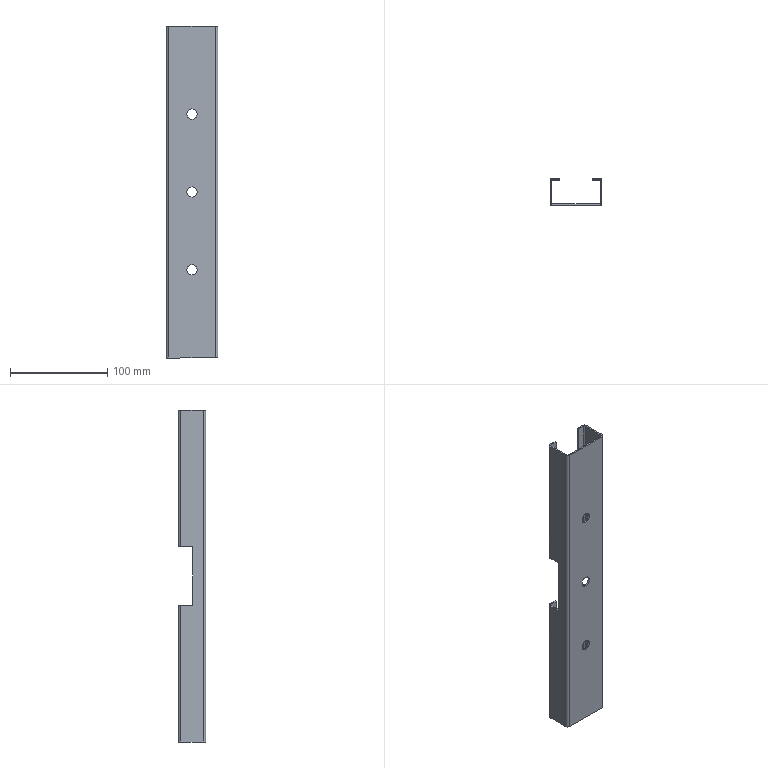Part | SolidWorks | features ICE 2, FlatPattern 1, SMBaseFlange 1, SheetMetal 1 | 1 solid | 68 faces | box 53 x 28 x 341 mm | volume 56893 mm3 | plane 50 | cylinder 18 | commonest cylinder face diameters 2 x6 5 x6 10.5 x6